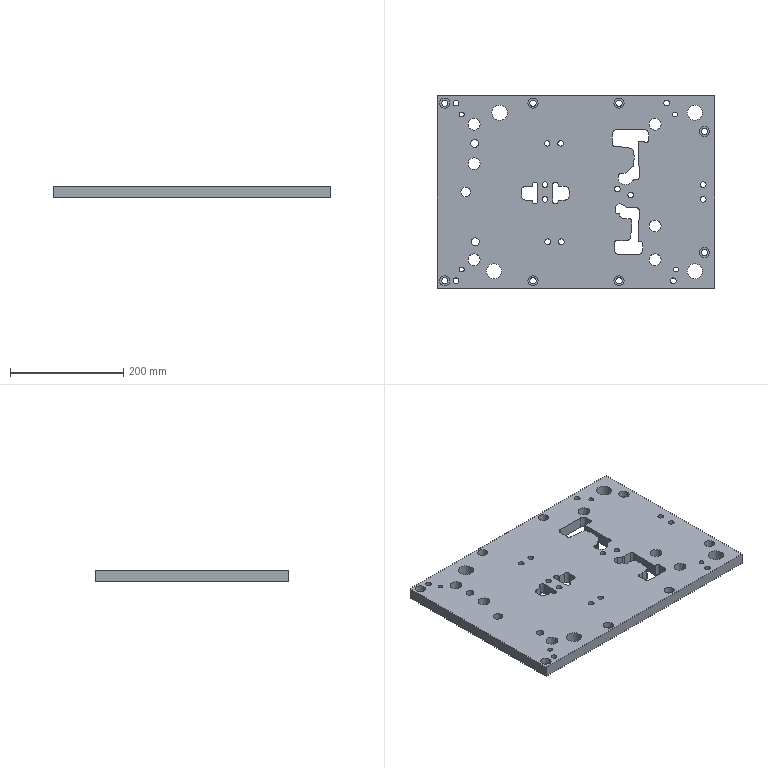Part | NX | features LIN_SOLID_COLOR 2 | 1 solid | 156 faces | box 490 x 340 x 20 mm | volume 3036614 mm3 | cylinder 84 | plane 72 | commonest cylinder face diameters 10 x19 2 x11 14 x10 11 x8 18 x8 21 x6